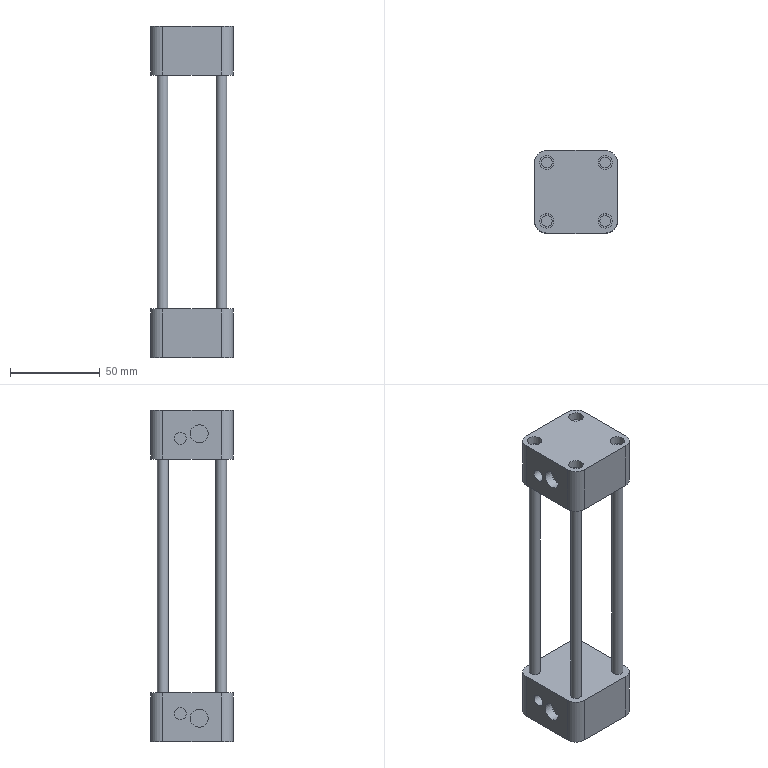Part | NX | features solid 2 | 1 solid | 48 faces | box 46 x 46 x 184 mm | volume 123684 mm3 | plane 24 | cylinder 24 | commonest cylinder face diameters 6 x8 13.5 x8 8 x4 6.667 x2 10 x2
STEP:
#1=CARTESIAN_POINT('',(-576.25,-3.,-304.));
#2=VERTEX_POINT('',#1);
#3=CARTESIAN_POINT('',(-543.75,-3.,-304.));
#4=VERTEX_POINT('',#3);
#5=CARTESIAN_POINT('',(-583.,-3.,-304.));
#6=DIRECTION('',(1.,0.,0.));
#7=VECTOR('',#6,1000.);
#8=LINE('',#5,#7);
#9=EDGE_CURVE('',#2,#4,#8,.T.);
#10=ORIENTED_EDGE('',*,*,#9,.F.);
#11=CARTESIAN_POINT('',(-576.25,-3.,-331.));
#12=VERTEX_POINT('',#11);
#13=CARTESIAN_POINT('',(-576.25,-3.,-331.));
#14=DIRECTION('',(0.,0.,-1.));
#15=VECTOR('',#14,1000.);
#16=LINE('',#13,#15);
#17=EDGE_CURVE('',#2,#12,#16,.T.);
#18=ORIENTED_EDGE('',*,*,#17,.T.);
#19=CARTESIAN_POINT('',(-543.75,-3.,-331.));
#20=VERTEX_POINT('',#19);
#21=CARTESIAN_POINT('',(-583.,-3.,-331.));
#22=DIRECTION('',(1.,0.,0.));
#23=VECTOR('',#22,1000.);
#24=LINE('',#21,#23);
#25=EDGE_CURVE('',#12,#20,#24,.T.);
#26=ORIENTED_EDGE('',*,*,#25,.T.);
#27=CARTESIAN_POINT('',(-543.75,-3.,-304.));
#28=DIRECTION('',(0.,0.,-1.));
#29=VECTOR('',#28,1000.);
#30=LINE('',#27,#29);
#31=EDGE_CURVE('',#20,#4,#30,.F.);
#32=ORIENTED_EDGE('',*,*,#31,.T.);
#33=EDGE_LOOP('',(#10,#18,#26,#32));
#34=FACE_BOUND('',#33,.T.);
#35=CARTESIAN_POINT('',(-583.,-3.,-304.));
#36=DIRECTION('',(0.,1.,0.));
#37=DIRECTION('',(-1.,0.,0.));
#38=AXIS2_PLACEMENT_3D('',#35,#36,#37);
#39=PLANE('',#38);
#40=ADVANCED_FACE('',(#34),#39,.F.);
#41=CARTESIAN_POINT('',(-537.,36.25,-304.));
#42=VERTEX_POINT('',#41);
#43=CARTESIAN_POINT('',(-537.,3.75,-304.));
#44=VERTEX_POINT('',#43);
#45=CARTESIAN_POINT('',(-537.,43.,-304.));
#46=DIRECTION('',(0.,-1.,0.));
#47=VECTOR('',#46,1000.);
#48=LINE('',#45,#47);
#49=EDGE_CURVE('',#42,#44,#48,.T.);
#50=ORIENTED_EDGE('',*,*,#49,.T.);
#51=CARTESIAN_POINT('',(-537.,3.75,-331.));
#52=VERTEX_POINT('',#51);
#53=CARTESIAN_POINT('',(-537.,3.75,-331.));
#54=DIRECTION('',(0.,0.,-1.));
#55=VECTOR('',#54,1000.);
#56=LINE('',#53,#55);
#57=EDGE_CURVE('',#44,#52,#56,.T.);
#58=ORIENTED_EDGE('',*,*,#57,.T.);
#59=CARTESIAN_POINT('',(-537.,36.25,-331.));
#60=VERTEX_POINT('',#59);
#61=CARTESIAN_POINT('',(-537.,43.,-331.));
#62=DIRECTION('',(0.,-1.,0.));
#63=VECTOR('',#62,1000.);
#64=LINE('',#61,#63);
#65=EDGE_CURVE('',#60,#52,#64,.T.);
#66=ORIENTED_EDGE('',*,*,#65,.F.);
#67=CARTESIAN_POINT('',(-537.,36.25,-304.));
#68=DIRECTION('',(0.,0.,-1.));
#69=VECTOR('',#68,1000.);
#70=LINE('',#67,#69);
#71=EDGE_CURVE('',#60,#42,#70,.F.);
#72=ORIENTED_EDGE('',*,*,#71,.T.);
#73=EDGE_LOOP('',(#50,#58,#66,#72));
#74=FACE_BOUND('',#73,.T.);
#75=CARTESIAN_POINT('',(-537.,43.,-304.));
#76=DIRECTION('',(1.,0.,0.));
#77=DIRECTION('',(0.,1.,0.));
#78=AXIS2_PLACEMENT_3D('',#75,#76,#77);
#79=PLANE('',#78);
#80=ADVANCED_FACE('',(#74),#79,.T.);
#81=CARTESIAN_POINT('',(-543.75,43.,-331.));
#82=VERTEX_POINT('',#81);
#83=CARTESIAN_POINT('',(-576.25,43.,-331.));
#84=VERTEX_POINT('',#83);
#85=CARTESIAN_POINT('',(-537.,43.,-331.));
#86=DIRECTION('',(-1.,0.,0.));
#87=VECTOR('',#86,1000.);
#88=LINE('',#85,#87);
#89=EDGE_CURVE('',#82,#84,#88,.T.);
#90=ORIENTED_EDGE('',*,*,#89,.T.);
#91=CARTESIAN_POINT('',(-576.25,43.,-304.));
#92=VERTEX_POINT('',#91);
#93=CARTESIAN_POINT('',(-576.25,43.,-304.));
#94=DIRECTION('',(0.,0.,-1.));
#95=VECTOR('',#94,1000.);
#96=LINE('',#93,#95);
#97=EDGE_CURVE('',#84,#92,#96,.F.);
#98=ORIENTED_EDGE('',*,*,#97,.T.);
#99=CARTESIAN_POINT('',(-543.75,43.,-304.));
#100=VERTEX_POINT('',#99);
#101=CARTESIAN_POINT('',(-537.,43.,-304.));
#102=DIRECTION('',(-1.,0.,0.));
#103=VECTOR('',#102,1000.);
#104=LINE('',#101,#103);
#105=EDGE_CURVE('',#100,#92,#104,.T.);
#106=ORIENTED_EDGE('',*,*,#105,.F.);
#107=CARTESIAN_POINT('',(-543.75,43.,-331.));
#108=DIRECTION('',(0.,0.,-1.));
#109=VECTOR('',#108,1000.);
#110=LINE('',#107,#109);
#111=EDGE_CURVE('',#100,#82,#110,.T.);
#112=ORIENTED_EDGE('',*,*,#111,.T.);
#113=EDGE_LOOP('',(#90,#98,#106,#112));
#114=FACE_BOUND('',#113,.T.);
#115=CARTESIAN_POINT('',(-537.,43.,-304.));
#116=DIRECTION('',(0.,-1.,0.));
#117=DIRECTION('',(1.,0.,0.));
#118=AXIS2_PLACEMENT_3D('',#115,#116,#117);
#119=PLANE('',#118);
#120=ADVANCED_FACE('',(#114),#119,.F.);
#121=CARTESIAN_POINT('',(-583.,26.5,-318.833));
#122=VERTEX_POINT('',#121);
#123=CARTESIAN_POINT('',(-583.,26.5,-315.5));
#124=DIRECTION('',(1.,0.,0.));
#125=DIRECTION('',(0.,0.,-1.));
#126=AXIS2_PLACEMENT_3D('',#123,#124,#125);
#127=CIRCLE('',#126,3.333);
#128=EDGE_CURVE('',#122,#122,#127,.T.);
#129=ORIENTED_EDGE('',*,*,#128,.T.);
#130=EDGE_LOOP('',(#129));
#131=FACE_BOUND('',#130,.T.);
#132=CARTESIAN_POINT('',(-583.,16.,-323.));
#133=VERTEX_POINT('',#132);
#134=CARTESIAN_POINT('',(-583.,16.,-318.));
#135=DIRECTION('',(1.,0.,0.));
#136=DIRECTION('',(0.,0.,-1.));
#137=AXIS2_PLACEMENT_3D('',#134,#135,#136);
#138=CIRCLE('',#137,5.);
#139=EDGE_CURVE('',#133,#133,#138,.T.);
#140=ORIENTED_EDGE('',*,*,#139,.T.);
#141=EDGE_LOOP('',(#140));
#142=FACE_BOUND('',#141,.T.);
#143=CARTESIAN_POINT('',(-583.,3.75,-331.));
#144=VERTEX_POINT('',#143);
#145=CARTESIAN_POINT('',(-583.,36.25,-331.));
#146=VERTEX_POINT('',#145);
#147=CARTESIAN_POINT('',(-583.,-3.,-331.));
#148=DIRECTION('',(0.,1.,0.));
#149=VECTOR('',#148,1000.);
#150=LINE('',#147,#149);
#151=EDGE_CURVE('',#144,#146,#150,.T.);
#152=ORIENTED_EDGE('',*,*,#151,.F.);
#153=CARTESIAN_POINT('',(-583.,3.75,-304.));
#154=VERTEX_POINT('',#153);
#155=CARTESIAN_POINT('',(-583.,3.75,-304.));
#156=DIRECTION('',(0.,0.,-1.));
#157=VECTOR('',#156,1000.);
#158=LINE('',#155,#157);
#159=EDGE_CURVE('',#144,#154,#158,.F.);
#160=ORIENTED_EDGE('',*,*,#159,.T.);
#161=CARTESIAN_POINT('',(-583.,36.25,-304.));
#162=VERTEX_POINT('',#161);
#163=CARTESIAN_POINT('',(-583.,-3.,-304.));
#164=DIRECTION('',(0.,1.,0.));
#165=VECTOR('',#164,1000.);
#166=LINE('',#163,#165);
#167=EDGE_CURVE('',#154,#162,#166,.T.);
#168=ORIENTED_EDGE('',*,*,#167,.T.);
#169=CARTESIAN_POINT('',(-583.,36.25,-331.));
#170=DIRECTION('',(0.,0.,-1.));
#171=VECTOR('',#170,1000.);
#172=LINE('',#169,#171);
#173=EDGE_CURVE('',#162,#146,#172,.T.);
#174=ORIENTED_EDGE('',*,*,#173,.T.);
#175=EDGE_LOOP('',(#152,#160,#168,#174));
#176=FACE_BOUND('',#175,.T.);
#177=CARTESIAN_POINT('',(-583.,-3.,-304.));
#178=DIRECTION('',(-1.,0.,0.));
#179=DIRECTION('',(0.,0.,1.));
#180=AXIS2_PLACEMENT_3D('',#177,#178,#179);
#181=PLANE('',#180);
#182=ADVANCED_FACE('',(#131,#142,#176),#181,.T.);
#183=CARTESIAN_POINT('',(-576.25,33.25,-304.));
#184=VERTEX_POINT('',#183);
#185=CARTESIAN_POINT('',(-576.25,36.25,-304.));
#186=DIRECTION('',(0.,0.,1.));
#187=DIRECTION('',(0.,-1.,0.));
#188=AXIS2_PLACEMENT_3D('',#185,#186,#187);
#189=CIRCLE('',#188,3.);
#190=EDGE_CURVE('',#184,#184,#189,.T.);
#191=ORIENTED_EDGE('',*,*,#190,.F.);
#192=EDGE_LOOP('',(#191));
#193=FACE_BOUND('',#192,.T.);
#194=CARTESIAN_POINT('',(-576.25,6.75,-304.));
#195=VERTEX_POINT('',#194);
#196=CARTESIAN_POINT('',(-576.25,3.75,-304.));
#197=DIRECTION('',(0.,0.,-1.));
#198=DIRECTION('',(0.,1.,0.));
#199=AXIS2_PLACEMENT_3D('',#196,#197,#198);
#200=CIRCLE('',#199,3.);
#201=EDGE_CURVE('',#195,#195,#200,.T.);
#202=ORIENTED_EDGE('',*,*,#201,.T.);
#203=EDGE_LOOP('',(#202));
#204=FACE_BOUND('',#203,.T.);
#205=CARTESIAN_POINT('',(-543.75,33.25,-304.));
#206=VERTEX_POINT('',#205);
#207=CARTESIAN_POINT('',(-543.75,36.25,-304.));
#208=DIRECTION('',(0.,0.,-1.));
#209=DIRECTION('',(0.,-1.,0.));
#210=AXIS2_PLACEMENT_3D('',#207,#208,#209);
#211=CIRCLE('',#210,3.);
#212=EDGE_CURVE('',#206,#206,#211,.T.);
#213=ORIENTED_EDGE('',*,*,#212,.T.);
#214=EDGE_LOOP('',(#213));
#215=FACE_BOUND('',#214,.T.);
#216=CARTESIAN_POINT('',(-543.75,6.75,-304.));
#217=VERTEX_POINT('',#216);
#218=CARTESIAN_POINT('',(-543.75,3.75,-304.));
#219=DIRECTION('',(0.,0.,1.));
#220=DIRECTION('',(0.,1.,0.));
#221=AXIS2_PLACEMENT_3D('',#218,#219,#220);
#222=CIRCLE('',#221,3.);
#223=EDGE_CURVE('',#217,#217,#222,.T.);
#224=ORIENTED_EDGE('',*,*,#223,.F.);
#225=EDGE_LOOP('',(#224));
#226=FACE_BOUND('',#225,.T.);
#227=ORIENTED_EDGE('',*,*,#167,.F.);
#228=CARTESIAN_POINT('',(-576.25,3.75,-304.));
#229=DIRECTION('',(0.,0.,-1.));
#230=DIRECTION('',(0.,-1.,0.));
#231=AXIS2_PLACEMENT_3D('',#228,#229,#230);
#232=CIRCLE('',#231,6.75);
#233=EDGE_CURVE('',#154,#2,#232,.F.);
#234=ORIENTED_EDGE('',*,*,#233,.T.);
#235=ORIENTED_EDGE('',*,*,#9,.T.);
#236=CARTESIAN_POINT('',(-543.75,3.75,-304.));
#237=DIRECTION('',(0.,0.,-1.));
#238=DIRECTION('',(0.,-1.,0.));
#239=AXIS2_PLACEMENT_3D('',#236,#237,#238);
#240=CIRCLE('',#239,6.75);
#241=EDGE_CURVE('',#4,#44,#240,.F.);
#242=ORIENTED_EDGE('',*,*,#241,.T.);
#243=ORIENTED_EDGE('',*,*,#49,.F.);
#244=CARTESIAN_POINT('',(-543.75,36.25,-304.));
#245=DIRECTION('',(0.,0.,-1.));
#246=DIRECTION('',(0.,-1.,0.));
#247=AXIS2_PLACEMENT_3D('',#244,#245,#246);
#248=CIRCLE('',#247,6.75);
#249=EDGE_CURVE('',#42,#100,#248,.F.);
#250=ORIENTED_EDGE('',*,*,#249,.T.);
#251=ORIENTED_EDGE('',*,*,#105,.T.);
#252=CARTESIAN_POINT('',(-576.25,36.25,-304.));
#253=DIRECTION('',(0.,0.,-1.));
#254=DIRECTION('',(0.,-1.,0.));
#255=AXIS2_PLACEMENT_3D('',#252,#253,#254);
#256=CIRCLE('',#255,6.75);
#257=EDGE_CURVE('',#92,#162,#256,.F.);
#258=ORIENTED_EDGE('',*,*,#257,.T.);
#259=EDGE_LOOP('',(#227,#234,#235,#242,#243,#250,#251,#258));
#260=FACE_BOUND('',#259,.T.);
#261=CARTESIAN_POINT('',(-537.,-3.,-304.));
#262=DIRECTION('',(0.,0.,-1.));
#263=DIRECTION('',(0.,-1.,0.));
#264=AXIS2_PLACEMENT_3D('',#261,#262,#263);
#265=PLANE('',#264);
#266=ADVANCED_FACE('',(#193,#204,#215,#226,#260),#265,.F.);
#267=ORIENTED_EDGE('',*,*,#25,.F.);
#268=CARTESIAN_POINT('',(-576.25,3.75,-331.));
#269=DIRECTION('',(0.,0.,-1.));
#270=DIRECTION('',(0.,-1.,0.));
#271=AXIS2_PLACEMENT_3D('',#268,#269,#270);
#272=CIRCLE('',#271,6.75);
#273=EDGE_CURVE('',#12,#144,#272,.T.);
#274=ORIENTED_EDGE('',*,*,#273,.T.);
#275=ORIENTED_EDGE('',*,*,#151,.T.);
#276=CARTESIAN_POINT('',(-576.25,36.25,-331.));
#277=DIRECTION('',(0.,0.,-1.));
#278=DIRECTION('',(0.,-1.,0.));
#279=AXIS2_PLACEMENT_3D('',#276,#277,#278);
#280=CIRCLE('',#279,6.75);
#281=EDGE_CURVE('',#146,#84,#280,.T.);
#282=ORIENTED_EDGE('',*,*,#281,.T.);
#283=ORIENTED_EDGE('',*,*,#89,.F.);
#284=CARTESIAN_POINT('',(-543.75,36.25,-331.));
#285=DIRECTION('',(0.,0.,-1.));
#286=DIRECTION('',(0.,-1.,0.));
#287=AXIS2_PLACEMENT_3D('',#284,#285,#286);
#288=CIRCLE('',#287,6.75);
#289=EDGE_CURVE('',#82,#60,#288,.T.);
#290=ORIENTED_EDGE('',*,*,#289,.T.);
#291=ORIENTED_EDGE('',*,*,#65,.T.);
#292=CARTESIAN_POINT('',(-543.75,3.75,-331.));
#293=DIRECTION('',(0.,0.,-1.));
#294=DIRECTION('',(0.,-1.,0.));
#295=AXIS2_PLACEMENT_3D('',#292,#293,#294);
#296=CIRCLE('',#295,6.75);
#297=EDGE_CURVE('',#52,#20,#296,.T.);
#298=ORIENTED_EDGE('',*,*,#297,.T.);
#299=EDGE_LOOP('',(#267,#274,#275,#282,#283,#290,#291,#298));
#300=FACE_BOUND('',#299,.T.);
#301=CARTESIAN_POINT('',(-537.,-3.,-331.));
#302=DIRECTION('',(0.,0.,-1.));
#303=DIRECTION('',(0.,-1.,0.));
#304=AXIS2_PLACEMENT_3D('',#301,#302,#303);
#305=PLANE('',#304);
#306=ADVANCED_FACE('',(#300),#305,.T.);
#307=ORIENTED_EDGE('',*,*,#233,.F.);
#308=ORIENTED_EDGE('',*,*,#159,.F.);
#309=ORIENTED_EDGE('',*,*,#273,.F.);
#310=ORIENTED_EDGE('',*,*,#17,.F.);
#311=EDGE_LOOP('',(#307,#308,#309,#310));
#312=FACE_BOUND('',#311,.T.);
#313=CARTESIAN_POINT('',(-576.25,3.75,-304.));
#314=DIRECTION('',(0.,0.,1.));
#315=DIRECTION('',(0.,1.,0.));
#316=AXIS2_PLACEMENT_3D('',#313,#314,#315);
#317=CYLINDRICAL_SURFACE('',#316,6.75);
#318=ADVANCED_FACE('',(#312),#317,.T.);
#319=ORIENTED_EDGE('',*,*,#241,.F.);
#320=ORIENTED_EDGE('',*,*,#31,.F.);
#321=ORIENTED_EDGE('',*,*,#297,.F.);
#322=ORIENTED_EDGE('',*,*,#57,.F.);
#323=EDGE_LOOP('',(#319,#320,#321,#322));
#324=FACE_BOUND('',#323,.T.);
#325=CARTESIAN_POINT('',(-543.75,3.75,-304.));
#326=DIRECTION('',(0.,0.,1.));
#327=DIRECTION('',(0.,1.,0.));
#328=AXIS2_PLACEMENT_3D('',#325,#326,#327);
#329=CYLINDRICAL_SURFACE('',#328,6.75);
#330=ADVANCED_FACE('',(#324),#329,.T.);
#331=ORIENTED_EDGE('',*,*,#257,.F.);
#332=ORIENTED_EDGE('',*,*,#97,.F.);
#333=ORIENTED_EDGE('',*,*,#281,.F.);
#334=ORIENTED_EDGE('',*,*,#173,.F.);
#335=EDGE_LOOP('',(#331,#332,#333,#334));
#336=FACE_BOUND('',#335,.T.);
#337=CARTESIAN_POINT('',(-576.25,36.25,-304.));
#338=DIRECTION('',(0.,0.,1.));
#339=DIRECTION('',(0.,1.,0.));
#340=AXIS2_PLACEMENT_3D('',#337,#338,#339);
#341=CYLINDRICAL_SURFACE('',#340,6.75);
#342=ADVANCED_FACE('',(#336),#341,.T.);
#343=ORIENTED_EDGE('',*,*,#249,.F.);
#344=ORIENTED_EDGE('',*,*,#71,.F.);
#345=ORIENTED_EDGE('',*,*,#289,.F.);
#346=ORIENTED_EDGE('',*,*,#111,.F.);
#347=EDGE_LOOP('',(#343,#344,#345,#346));
#348=FACE_BOUND('',#347,.T.);
#349=CARTESIAN_POINT('',(-543.75,36.25,-304.));
#350=DIRECTION('',(0.,0.,1.));
#351=DIRECTION('',(0.,1.,0.));
#352=AXIS2_PLACEMENT_3D('',#349,#350,#351);
#353=CYLINDRICAL_SURFACE('',#352,6.75);
#354=ADVANCED_FACE('',(#348),#353,.T.);
#355=CARTESIAN_POINT('',(-543.75,0.75,-174.));
#356=VERTEX_POINT('',#355);
#357=CARTESIAN_POINT('',(-543.75,3.75,-174.));
#358=DIRECTION('',(0.,0.,-1.));
#359=DIRECTION('',(0.,-1.,0.));
#360=AXIS2_PLACEMENT_3D('',#357,#358,#359);
#361=CIRCLE('',#360,3.);
#362=EDGE_CURVE('',#356,#356,#361,.F.);
#363=ORIENTED_EDGE('',*,*,#362,.F.);
#364=EDGE_LOOP('',(#363));
#365=FACE_BOUND('',#364,.T.);
#366=ORIENTED_EDGE('',*,*,#223,.T.);
#367=EDGE_LOOP('',(#366));
#368=FACE_BOUND('',#367,.T.);
#369=CARTESIAN_POINT('',(-543.75,3.75,-304.));
#370=DIRECTION('',(0.,0.,1.));
#371=DIRECTION('',(0.,1.,0.));
#372=AXIS2_PLACEMENT_3D('',#369,#370,#371);
#373=CYLINDRICAL_SURFACE('',#372,3.);
#374=ADVANCED_FACE('',(#365,#368),#373,.T.);
#375=CARTESIAN_POINT('',(-543.75,33.25,-174.));
#376=VERTEX_POINT('',#375);
#377=CARTESIAN_POINT('',(-543.75,36.25,-174.));
#378=DIRECTION('',(0.,0.,-1.));
#379=DIRECTION('',(0.,-1.,0.));
#380=AXIS2_PLACEMENT_3D('',#377,#378,#379);
#381=CIRCLE('',#380,3.);
#382=EDGE_CURVE('',#376,#376,#381,.F.);
#383=ORIENTED_EDGE('',*,*,#382,.F.);
#384=EDGE_LOOP('',(#383));
#385=FACE_BOUND('',#384,.T.);
#386=ORIENTED_EDGE('',*,*,#212,.F.);
#387=EDGE_LOOP('',(#386));
#388=FACE_BOUND('',#387,.T.);
#389=CARTESIAN_POINT('',(-543.75,36.25,-304.));
#390=DIRECTION('',(0.,0.,1.));
#391=DIRECTION('',(0.,-1.,0.));
#392=AXIS2_PLACEMENT_3D('',#389,#390,#391);
#393=CYLINDRICAL_SURFACE('',#392,3.);
#394=ADVANCED_FACE('',(#385,#388),#393,.T.);
#395=CARTESIAN_POINT('',(-576.25,0.75,-174.));
#396=VERTEX_POINT('',#395);
#397=CARTESIAN_POINT('',(-576.25,3.75,-174.));
#398=DIRECTION('',(0.,0.,-1.));
#399=DIRECTION('',(0.,-1.,0.));
#400=AXIS2_PLACEMENT_3D('',#397,#398,#399);
#401=CIRCLE('',#400,3.);
#402=EDGE_CURVE('',#396,#396,#401,.F.);
#403=ORIENTED_EDGE('',*,*,#402,.F.);
#404=EDGE_LOOP('',(#403));
#405=FACE_BOUND('',#404,.T.);
#406=ORIENTED_EDGE('',*,*,#201,.F.);
#407=EDGE_LOOP('',(#406));
#408=FACE_BOUND('',#407,.T.);
#409=CARTESIAN_POINT('',(-576.25,3.75,-304.));
#410=DIRECTION('',(0.,0.,1.));
#411=DIRECTION('',(0.,1.,0.));
#412=AXIS2_PLACEMENT_3D('',#409,#410,#411);
#413=CYLINDRICAL_SURFACE('',#412,3.);
#414=ADVANCED_FACE('',(#405,#408),#413,.T.);
#415=CARTESIAN_POINT('',(-576.25,33.25,-174.));
#416=VERTEX_POINT('',#415);
#417=CARTESIAN_POINT('',(-576.25,36.25,-174.));
#418=DIRECTION('',(0.,0.,-1.));
#419=DIRECTION('',(0.,-1.,0.));
#420=AXIS2_PLACEMENT_3D('',#417,#418,#419);
#421=CIRCLE('',#420,3.);
#422=EDGE_CURVE('',#416,#416,#421,.F.);
#423=ORIENTED_EDGE('',*,*,#422,.F.);
#424=EDGE_LOOP('',(#423));
#425=FACE_BOUND('',#424,.T.);
#426=ORIENTED_EDGE('',*,*,#190,.T.);
#427=EDGE_LOOP('',(#426));
#428=FACE_BOUND('',#427,.T.);
#429=CARTESIAN_POINT('',(-576.25,36.25,-304.));
#430=DIRECTION('',(0.,0.,1.));
#431=DIRECTION('',(0.,-1.,0.));
#432=AXIS2_PLACEMENT_3D('',#429,#430,#431);
#433=CYLINDRICAL_SURFACE('',#432,3.);
#434=ADVANCED_FACE('',(#425,#428),#433,.T.);
#435=CARTESIAN_POINT('',(-578.,16.,-323.));
#436=VERTEX_POINT('',#435);
#437=CARTESIAN_POINT('',(-578.,16.,-318.));
#438=DIRECTION('',(1.,0.,0.));
#439=DIRECTION('',(0.,0.,-1.));
#440=AXIS2_PLACEMENT_3D('',#437,#438,#439);
#441=CIRCLE('',#440,5.);
#442=EDGE_CURVE('',#436,#436,#441,.T.);
#443=ORIENTED_EDGE('',*,*,#442,.F.);
#444=EDGE_LOOP('',(#443));
#445=FACE_BOUND('',#444,.T.);
#446=CARTESIAN_POINT('',(-578.,16.,-318.));
#447=DIRECTION('',(1.,0.,0.));
#448=DIRECTION('',(0.,0.,-1.));
#449=AXIS2_PLACEMENT_3D('',#446,#447,#448);
#450=PLANE('',#449);
#451=ADVANCED_FACE('',(#445),#450,.F.);
#452=ORIENTED_EDGE('',*,*,#442,.T.);
#453=EDGE_LOOP('',(#452));
#454=FACE_BOUND('',#453,.T.);
#455=ORIENTED_EDGE('',*,*,#139,.F.);
#456=EDGE_LOOP('',(#455));
#457=FACE_BOUND('',#456,.T.);
#458=CARTESIAN_POINT('',(-583.,16.,-318.));
#459=DIRECTION('',(1.,0.,0.));
#460=DIRECTION('',(0.,0.,-1.));
#461=AXIS2_PLACEMENT_3D('',#458,#459,#460);
#462=CYLINDRICAL_SURFACE('',#461,5.);
#463=ADVANCED_FACE('',(#454,#457),#462,.F.);
#464=CARTESIAN_POINT('',(-578.,26.5,-318.833));
#465=VERTEX_POINT('',#464);
#466=CARTESIAN_POINT('',(-578.,26.5,-315.5));
#467=DIRECTION('',(1.,0.,0.));
#468=DIRECTION('',(0.,0.,-1.));
#469=AXIS2_PLACEMENT_3D('',#466,#467,#468);
#470=CIRCLE('',#469,3.333);
#471=EDGE_CURVE('',#465,#465,#470,.T.);
#472=ORIENTED_EDGE('',*,*,#471,.F.);
#473=EDGE_LOOP('',(#472));
#474=FACE_BOUND('',#473,.T.);
#475=CARTESIAN_POINT('',(-578.,26.5,-315.5));
#476=DIRECTION('',(1.,0.,0.));
#477=DIRECTION('',(0.,0.,-1.));
#478=AXIS2_PLACEMENT_3D('',#475,#476,#477);
#479=PLANE('',#478);
#480=ADVANCED_FACE('',(#474),#479,.F.);
#481=ORIENTED_EDGE('',*,*,#471,.T.);
#482=EDGE_LOOP('',(#481));
#483=FACE_BOUND('',#482,.T.);
#484=ORIENTED_EDGE('',*,*,#128,.F.);
#485=EDGE_LOOP('',(#484));
#486=FACE_BOUND('',#485,.T.);
#487=CARTESIAN_POINT('',(-583.,26.5,-315.5));
#488=DIRECTION('',(1.,0.,0.));
#489=DIRECTION('',(0.,0.,-1.));
#490=AXIS2_PLACEMENT_3D('',#487,#488,#489);
#491=CYLINDRICAL_SURFACE('',#490,3.333);
#492=ADVANCED_FACE('',(#483,#486),#491,.F.);
#493=CARTESIAN_POINT('',(-543.75,43.,-174.));
#494=VERTEX_POINT('',#493);
#495=CARTESIAN_POINT('',(-576.25,43.,-174.));
#496=VERTEX_POINT('',#495);
#497=CARTESIAN_POINT('',(-537.,43.,-174.));
#498=DIRECTION('',(-1.,0.,0.));
#499=VECTOR('',#498,1000.);
#500=LINE('',#497,#499);
#501=EDGE_CURVE('',#494,#496,#500,.T.);
#502=ORIENTED_EDGE('',*,*,#501,.T.);
#503=CARTESIAN_POINT('',(-576.25,43.,-147.));
#504=VERTEX_POINT('',#503);
#505=CARTESIAN_POINT('',(-576.25,43.,-147.));
#506=DIRECTION('',(0.,0.,1.));
#507=VECTOR('',#506,1000.);
#508=LINE('',#505,#507);
#509=EDGE_CURVE('',#496,#504,#508,.T.);
#510=ORIENTED_EDGE('',*,*,#509,.T.);
#511=CARTESIAN_POINT('',(-543.75,43.,-147.));
#512=VERTEX_POINT('',#511);
#513=CARTESIAN_POINT('',(-537.,43.,-147.));
#514=DIRECTION('',(-1.,0.,0.));
#515=VECTOR('',#514,1000.);
#516=LINE('',#513,#515);
#517=EDGE_CURVE('',#512,#504,#516,.T.);
#518=ORIENTED_EDGE('',*,*,#517,.F.);
#519=CARTESIAN_POINT('',(-543.75,43.,-174.));
#520=DIRECTION('',(0.,0.,1.));
#521=VECTOR('',#520,1000.);
#522=LINE('',#519,#521);
#523=EDGE_CURVE('',#512,#494,#522,.F.);
#524=ORIENTED_EDGE('',*,*,#523,.T.);
#525=EDGE_LOOP('',(#502,#510,#518,#524));
#526=FACE_BOUND('',#525,.T.);
#527=CARTESIAN_POINT('',(-537.,43.,-174.));
#528=DIRECTION('',(0.,1.,0.));
#529=DIRECTION('',(-1.,0.,0.));
#530=AXIS2_PLACEMENT_3D('',#527,#528,#529);
#531=PLANE('',#530);
#532=ADVANCED_FACE('',(#526),#531,.T.);
#533=CARTESIAN_POINT('',(-583.,26.5,-165.833));
#534=VERTEX_POINT('',#533);
#535=CARTESIAN_POINT('',(-583.,26.5,-162.5));
#536=DIRECTION('',(1.,0.,0.));
#537=DIRECTION('',(0.,0.,-1.));
#538=AXIS2_PLACEMENT_3D('',#535,#536,#537);
#539=CIRCLE('',#538,3.333);
#540=EDGE_CURVE('',#534,#534,#539,.T.);
#541=ORIENTED_EDGE('',*,*,#540,.T.);
#542=EDGE_LOOP('',(#541));
#543=FACE_BOUND('',#542,.T.);
#544=CARTESIAN_POINT('',(-583.,16.,-165.));
#545=VERTEX_POINT('',#544);
#546=CARTESIAN_POINT('',(-583.,16.,-160.));
#547=DIRECTION('',(1.,0.,0.));
#548=DIRECTION('',(0.,0.,-1.));
#549=AXIS2_PLACEMENT_3D('',#546,#547,#548);
#550=CIRCLE('',#549,5.);
#551=EDGE_CURVE('',#545,#545,#550,.T.);
#552=ORIENTED_EDGE('',*,*,#551,.T.);
#553=EDGE_LOOP('',(#552));
#554=FACE_BOUND('',#553,.T.);
#555=CARTESIAN_POINT('',(-583.,3.75,-147.));
#556=VERTEX_POINT('',#555);
#557=CARTESIAN_POINT('',(-583.,36.25,-147.));
#558=VERTEX_POINT('',#557);
#559=CARTESIAN_POINT('',(-583.,-3.,-147.));
#560=DIRECTION('',(0.,1.,0.));
#561=VECTOR('',#560,1000.);
#562=LINE('',#559,#561);
#563=EDGE_CURVE('',#556,#558,#562,.T.);
#564=ORIENTED_EDGE('',*,*,#563,.T.);
#565=CARTESIAN_POINT('',(-583.,36.25,-174.));
#566=VERTEX_POINT('',#565);
#567=CARTESIAN_POINT('',(-583.,36.25,-174.));
#568=DIRECTION('',(0.,0.,1.));
#569=VECTOR('',#568,1000.);
#570=LINE('',#567,#569);
#571=EDGE_CURVE('',#558,#566,#570,.F.);
#572=ORIENTED_EDGE('',*,*,#571,.T.);
#573=CARTESIAN_POINT('',(-583.,3.75,-174.));
#574=VERTEX_POINT('',#573);
#575=CARTESIAN_POINT('',(-583.,-3.,-174.));
#576=DIRECTION('',(0.,1.,0.));
#577=VECTOR('',#576,1000.);
#578=LINE('',#575,#577);
#579=EDGE_CURVE('',#574,#566,#578,.T.);
#580=ORIENTED_EDGE('',*,*,#579,.F.);
#581=CARTESIAN_POINT('',(-583.,3.75,-147.));
#582=DIRECTION('',(0.,0.,1.));
#583=VECTOR('',#582,1000.);
#584=LINE('',#581,#583);
#585=EDGE_CURVE('',#574,#556,#584,.T.);
#586=ORIENTED_EDGE('',*,*,#585,.T.);
#587=EDGE_LOOP('',(#564,#572,#580,#586));
#588=FACE_BOUND('',#587,.T.);
#589=CARTESIAN_POINT('',(-583.,-3.,-174.));
#590=DIRECTION('',(1.,0.,0.));
#591=DIRECTION('',(0.,0.,-1.));
#592=AXIS2_PLACEMENT_3D('',#589,#590,#591);
#593=PLANE('',#592);
#594=ADVANCED_FACE('',(#543,#554,#588),#593,.F.);
#595=CARTESIAN_POINT('',(-576.25,-3.,-174.));
#596=VERTEX_POINT('',#595);
#597=CARTESIAN_POINT('',(-543.75,-3.,-174.));
#598=VERTEX_POINT('',#597);
#599=CARTESIAN_POINT('',(-583.,-3.,-174.));
#600=DIRECTION('',(1.,0.,0.));
#601=VECTOR('',#600,1000.);
#602=LINE('',#599,#601);
#603=EDGE_CURVE('',#596,#598,#602,.T.);
#604=ORIENTED_EDGE('',*,*,#603,.T.);
#605=CARTESIAN_POINT('',(-543.75,-3.,-147.));
#606=VERTEX_POINT('',#605);
#607=CARTESIAN_POINT('',(-543.75,-3.,-147.));
#608=DIRECTION('',(0.,0.,1.));
#609=VECTOR('',#608,1000.);
#610=LINE('',#607,#609);
#611=EDGE_CURVE('',#598,#606,#610,.T.);
#612=ORIENTED_EDGE('',*,*,#611,.T.);
#613=CARTESIAN_POINT('',(-576.25,-3.,-147.));
#614=VERTEX_POINT('',#613);
#615=CARTESIAN_POINT('',(-583.,-3.,-147.));
#616=DIRECTION('',(1.,0.,0.));
#617=VECTOR('',#616,1000.);
#618=LINE('',#615,#617);
#619=EDGE_CURVE('',#614,#606,#618,.T.);
#620=ORIENTED_EDGE('',*,*,#619,.F.);
#621=CARTESIAN_POINT('',(-576.25,-3.,-174.));
#622=DIRECTION('',(0.,0.,1.));
#623=VECTOR('',#622,1000.);
#624=LINE('',#621,#623);
#625=EDGE_CURVE('',#614,#596,#624,.F.);
#626=ORIENTED_EDGE('',*,*,#625,.T.);
#627=EDGE_LOOP('',(#604,#612,#620,#626));
#628=FACE_BOUND('',#627,.T.);
#629=CARTESIAN_POINT('',(-583.,-3.,-174.));
#630=DIRECTION('',(0.,-1.,0.));
#631=DIRECTION('',(1.,0.,0.));
#632=AXIS2_PLACEMENT_3D('',#629,#630,#631);
#633=PLANE('',#632);
#634=ADVANCED_FACE('',(#628),#633,.T.);
#635=CARTESIAN_POINT('',(-537.,36.25,-174.));
#636=VERTEX_POINT('',#635);
#637=CARTESIAN_POINT('',(-537.,3.75,-174.));
#638=VERTEX_POINT('',#637);
#639=CARTESIAN_POINT('',(-537.,43.,-174.));
#640=DIRECTION('',(0.,-1.,0.));
#641=VECTOR('',#640,1000.);
#642=LINE('',#639,#641);
#643=EDGE_CURVE('',#636,#638,#642,.T.);
#644=ORIENTED_EDGE('',*,*,#643,.F.);
#645=CARTESIAN_POINT('',(-537.,36.25,-147.));
#646=VERTEX_POINT('',#645);
#647=CARTESIAN_POINT('',(-537.,36.25,-147.));
#648=DIRECTION('',(0.,0.,1.));
#649=VECTOR('',#648,1000.);
#650=LINE('',#647,#649);
#651=EDGE_CURVE('',#636,#646,#650,.T.);
#652=ORIENTED_EDGE('',*,*,#651,.T.);
#653=CARTESIAN_POINT('',(-537.,3.75,-147.));
#654=VERTEX_POINT('',#653);
#655=CARTESIAN_POINT('',(-537.,43.,-147.));
#656=DIRECTION('',(0.,-1.,0.));
#657=VECTOR('',#656,1000.);
#658=LINE('',#655,#657);
#659=EDGE_CURVE('',#646,#654,#658,.T.);
#660=ORIENTED_EDGE('',*,*,#659,.T.);
#661=CARTESIAN_POINT('',(-537.,3.75,-174.));
#662=DIRECTION('',(0.,0.,1.));
#663=VECTOR('',#662,1000.);
#664=LINE('',#661,#663);
#665=EDGE_CURVE('',#654,#638,#664,.F.);
#666=ORIENTED_EDGE('',*,*,#665,.T.);
#667=EDGE_LOOP('',(#644,#652,#660,#666));
#668=FACE_BOUND('',#667,.T.);
#669=CARTESIAN_POINT('',(-537.,43.,-174.));
#670=DIRECTION('',(-1.,0.,0.));
#671=DIRECTION('',(0.,-1.,0.));
#672=AXIS2_PLACEMENT_3D('',#669,#670,#671);
#673=PLANE('',#672);
#674=ADVANCED_FACE('',(#668),#673,.F.);
#675=ORIENTED_EDGE('',*,*,#362,.T.);
#676=EDGE_LOOP('',(#675));
#677=FACE_BOUND('',#676,.T.);
#678=ORIENTED_EDGE('',*,*,#382,.T.);
#679=EDGE_LOOP('',(#678));
#680=FACE_BOUND('',#679,.T.);
#681=ORIENTED_EDGE('',*,*,#402,.T.);
#682=EDGE_LOOP('',(#681));
#683=FACE_BOUND('',#682,.T.);
#684=ORIENTED_EDGE('',*,*,#422,.T.);
#685=EDGE_LOOP('',(#684));
#686=FACE_BOUND('',#685,.T.);
#687=ORIENTED_EDGE('',*,*,#579,.T.);
#688=CARTESIAN_POINT('',(-576.25,36.25,-174.));
#689=DIRECTION('',(0.,0.,-1.));
#690=DIRECTION('',(0.,-1.,0.));
#691=AXIS2_PLACEMENT_3D('',#688,#689,#690);
#692=CIRCLE('',#691,6.75);
#693=EDGE_CURVE('',#566,#496,#692,.T.);
#694=ORIENTED_EDGE('',*,*,#693,.T.);
#695=ORIENTED_EDGE('',*,*,#501,.F.);
#696=CARTESIAN_POINT('',(-543.75,36.25,-174.));
#697=DIRECTION('',(0.,0.,-1.));
#698=DIRECTION('',(0.,-1.,0.));
#699=AXIS2_PLACEMENT_3D('',#696,#697,#698);
#700=CIRCLE('',#699,6.75);
#701=EDGE_CURVE('',#494,#636,#700,.T.);
#702=ORIENTED_EDGE('',*,*,#701,.T.);
#703=ORIENTED_EDGE('',*,*,#643,.T.);
#704=CARTESIAN_POINT('',(-543.75,3.75,-174.));
#705=DIRECTION('',(0.,0.,-1.));
#706=DIRECTION('',(0.,-1.,0.));
#707=AXIS2_PLACEMENT_3D('',#704,#705,#706);
#708=CIRCLE('',#707,6.75);
#709=EDGE_CURVE('',#638,#598,#708,.T.);
#710=ORIENTED_EDGE('',*,*,#709,.T.);
#711=ORIENTED_EDGE('',*,*,#603,.F.);
#712=CARTESIAN_POINT('',(-576.25,3.75,-174.));
#713=DIRECTION('',(0.,0.,-1.));
#714=DIRECTION('',(0.,-1.,0.));
#715=AXIS2_PLACEMENT_3D('',#712,#713,#714);
#716=CIRCLE('',#715,6.75);
#717=EDGE_CURVE('',#596,#574,#716,.T.);
#718=ORIENTED_EDGE('',*,*,#717,.T.);
#719=EDGE_LOOP('',(#687,#694,#695,#702,#703,#710,#711,#718));
#720=FACE_BOUND('',#719,.T.);
#721=CARTESIAN_POINT('',(-583.,43.,-174.));
#722=DIRECTION('',(0.,0.,-1.));
#723=DIRECTION('',(0.,-1.,0.));
#724=AXIS2_PLACEMENT_3D('',#721,#722,#723);
#725=PLANE('',#724);
#726=ADVANCED_FACE('',(#677,#680,#683,#686,#720),#725,.T.);
#727=CARTESIAN_POINT('',(-543.75,7.75,-147.));
#728=VERTEX_POINT('',#727);
#729=CARTESIAN_POINT('',(-543.75,3.75,-147.));
#730=DIRECTION('',(0.,0.,-1.));
#731=DIRECTION('',(0.,1.,0.));
#732=AXIS2_PLACEMENT_3D('',#729,#730,#731);
#733=CIRCLE('',#732,4.);
#734=EDGE_CURVE('',#728,#728,#733,.T.);
#735=ORIENTED_EDGE('',*,*,#734,.T.);
#736=EDGE_LOOP('',(#735));
#737=FACE_BOUND('',#736,.T.);
#738=CARTESIAN_POINT('',(-576.25,7.75,-147.));
#739=VERTEX_POINT('',#738);
#740=CARTESIAN_POINT('',(-576.25,3.75,-147.));
#741=DIRECTION('',(0.,0.,1.));
#742=DIRECTION('',(0.,1.,0.));
#743=AXIS2_PLACEMENT_3D('',#740,#741,#742);
#744=CIRCLE('',#743,4.);
#745=EDGE_CURVE('',#739,#739,#744,.T.);
#746=ORIENTED_EDGE('',*,*,#745,.F.);
#747=EDGE_LOOP('',(#746));
#748=FACE_BOUND('',#747,.T.);
#749=CARTESIAN_POINT('',(-543.75,32.25,-147.));
#750=VERTEX_POINT('',#749);
#751=CARTESIAN_POINT('',(-543.75,36.25,-147.));
#752=DIRECTION('',(0.,0.,1.));
#753=DIRECTION('',(0.,-1.,0.));
#754=AXIS2_PLACEMENT_3D('',#751,#752,#753);
#755=CIRCLE('',#754,4.);
#756=EDGE_CURVE('',#750,#750,#755,.T.);
#757=ORIENTED_EDGE('',*,*,#756,.F.);
#758=EDGE_LOOP('',(#757));
#759=FACE_BOUND('',#758,.T.);
#760=CARTESIAN_POINT('',(-576.25,32.25,-147.));
#761=VERTEX_POINT('',#760);
#762=CARTESIAN_POINT('',(-576.25,36.25,-147.));
#763=DIRECTION('',(0.,0.,-1.));
#764=DIRECTION('',(0.,-1.,0.));
#765=AXIS2_PLACEMENT_3D('',#762,#763,#764);
#766=CIRCLE('',#765,4.);
#767=EDGE_CURVE('',#761,#761,#766,.T.);
#768=ORIENTED_EDGE('',*,*,#767,.T.);
#769=EDGE_LOOP('',(#768));
#770=FACE_BOUND('',#769,.T.);
#771=ORIENTED_EDGE('',*,*,#517,.T.);
#772=CARTESIAN_POINT('',(-576.25,36.25,-147.));
#773=DIRECTION('',(0.,0.,-1.));
#774=DIRECTION('',(0.,-1.,0.));
#775=AXIS2_PLACEMENT_3D('',#772,#773,#774);
#776=CIRCLE('',#775,6.75);
#777=EDGE_CURVE('',#504,#558,#776,.F.);
#778=ORIENTED_EDGE('',*,*,#777,.T.);
#779=ORIENTED_EDGE('',*,*,#563,.F.);
#780=CARTESIAN_POINT('',(-576.25,3.75,-147.));
#781=DIRECTION('',(0.,0.,-1.));
#782=DIRECTION('',(0.,-1.,0.));
#783=AXIS2_PLACEMENT_3D('',#780,#781,#782);
#784=CIRCLE('',#783,6.75);
#785=EDGE_CURVE('',#556,#614,#784,.F.);
#786=ORIENTED_EDGE('',*,*,#785,.T.);
#787=ORIENTED_EDGE('',*,*,#619,.T.);
#788=CARTESIAN_POINT('',(-543.75,3.75,-147.));
#789=DIRECTION('',(0.,0.,-1.));
#790=DIRECTION('',(0.,-1.,0.));
#791=AXIS2_PLACEMENT_3D('',#788,#789,#790);
#792=CIRCLE('',#791,6.75);
#793=EDGE_CURVE('',#606,#654,#792,.F.);
#794=ORIENTED_EDGE('',*,*,#793,.T.);
#795=ORIENTED_EDGE('',*,*,#659,.F.);
#796=CARTESIAN_POINT('',(-543.75,36.25,-147.));
#797=DIRECTION('',(0.,0.,-1.));
#798=DIRECTION('',(0.,-1.,0.));
#799=AXIS2_PLACEMENT_3D('',#796,#797,#798);
#800=CIRCLE('',#799,6.75);
#801=EDGE_CURVE('',#646,#512,#800,.F.);
#802=ORIENTED_EDGE('',*,*,#801,.T.);
#803=EDGE_LOOP('',(#771,#778,#779,#786,#787,#794,#795,#802));
#804=FACE_BOUND('',#803,.T.);
#805=CARTESIAN_POINT('',(-583.,43.,-147.));
#806=DIRECTION('',(0.,0.,-1.));
#807=DIRECTION('',(0.,-1.,0.));
#808=AXIS2_PLACEMENT_3D('',#805,#806,#807);
#809=PLANE('',#808);
#810=ADVANCED_FACE('',(#737,#748,#759,#770,#804),#809,.F.);
#811=ORIENTED_EDGE('',*,*,#693,.F.);
#812=ORIENTED_EDGE('',*,*,#571,.F.);
#813=ORIENTED_EDGE('',*,*,#777,.F.);
#814=ORIENTED_EDGE('',*,*,#509,.F.);
#815=EDGE_LOOP('',(#811,#812,#813,#814));
#816=FACE_BOUND('',#815,.T.);
#817=CARTESIAN_POINT('',(-576.25,36.25,-174.));
#818=DIRECTION('',(0.,0.,-1.));
#819=DIRECTION('',(0.,-1.,0.));
#820=AXIS2_PLACEMENT_3D('',#817,#818,#819);
#821=CYLINDRICAL_SURFACE('',#820,6.75);
#822=ADVANCED_FACE('',(#816),#821,.T.);
#823=ORIENTED_EDGE('',*,*,#701,.F.);
#824=ORIENTED_EDGE('',*,*,#523,.F.);
#825=ORIENTED_EDGE('',*,*,#801,.F.);
#826=ORIENTED_EDGE('',*,*,#651,.F.);
#827=EDGE_LOOP('',(#823,#824,#825,#826));
#828=FACE_BOUND('',#827,.T.);
#829=CARTESIAN_POINT('',(-543.75,36.25,-174.));
#830=DIRECTION('',(0.,0.,-1.));
#831=DIRECTION('',(0.,-1.,0.));
#832=AXIS2_PLACEMENT_3D('',#829,#830,#831);
#833=CYLINDRICAL_SURFACE('',#832,6.75);
#834=ADVANCED_FACE('',(#828),#833,.T.);
#835=ORIENTED_EDGE('',*,*,#709,.F.);
#836=ORIENTED_EDGE('',*,*,#665,.F.);
#837=ORIENTED_EDGE('',*,*,#793,.F.);
#838=ORIENTED_EDGE('',*,*,#611,.F.);
#839=EDGE_LOOP('',(#835,#836,#837,#838));
#840=FACE_BOUND('',#839,.T.);
#841=CARTESIAN_POINT('',(-543.75,3.75,-174.));
#842=DIRECTION('',(0.,0.,-1.));
#843=DIRECTION('',(0.,-1.,0.));
#844=AXIS2_PLACEMENT_3D('',#841,#842,#843);
#845=CYLINDRICAL_SURFACE('',#844,6.75);
#846=ADVANCED_FACE('',(#840),#845,.T.);
#847=ORIENTED_EDGE('',*,*,#717,.F.);
#848=ORIENTED_EDGE('',*,*,#625,.F.);
#849=ORIENTED_EDGE('',*,*,#785,.F.);
#850=ORIENTED_EDGE('',*,*,#585,.F.);
#851=EDGE_LOOP('',(#847,#848,#849,#850));
#852=FACE_BOUND('',#851,.T.);
#853=CARTESIAN_POINT('',(-576.25,3.75,-174.));
#854=DIRECTION('',(0.,0.,-1.));
#855=DIRECTION('',(0.,-1.,0.));
#856=AXIS2_PLACEMENT_3D('',#853,#854,#855);
#857=CYLINDRICAL_SURFACE('',#856,6.75);
#858=ADVANCED_FACE('',(#852),#857,.T.);
#859=CARTESIAN_POINT('',(-576.25,33.25,-165.));
#860=VERTEX_POINT('',#859);
#861=CARTESIAN_POINT('',(-576.25,36.25,-165.));
#862=DIRECTION('',(0.,0.,-1.));
#863=DIRECTION('',(0.,-1.,0.));
#864=AXIS2_PLACEMENT_3D('',#861,#862,#863);
#865=CIRCLE('',#864,3.);
#866=EDGE_CURVE('',#860,#860,#865,.F.);
#867=ORIENTED_EDGE('',*,*,#866,.F.);
#868=EDGE_LOOP('',(#867));
#869=FACE_BOUND('',#868,.T.);
#870=CARTESIAN_POINT('',(-576.25,32.25,-165.));
#871=VERTEX_POINT('',#870);
#872=CARTESIAN_POINT('',(-576.25,36.25,-165.));
#873=DIRECTION('',(0.,0.,-1.));
#874=DIRECTION('',(0.,-1.,0.));
#875=AXIS2_PLACEMENT_3D('',#872,#873,#874);
#876=CIRCLE('',#875,4.);
#877=EDGE_CURVE('',#871,#871,#876,.T.);
#878=ORIENTED_EDGE('',*,*,#877,.F.);
#879=EDGE_LOOP('',(#878));
#880=FACE_BOUND('',#879,.T.);
#881=CARTESIAN_POINT('',(-576.25,36.25,-165.));
#882=DIRECTION('',(0.,0.,-1.));
#883=DIRECTION('',(0.,-1.,0.));
#884=AXIS2_PLACEMENT_3D('',#881,#882,#883);
#885=PLANE('',#884);
#886=ADVANCED_FACE('',(#869,#880),#885,.F.);
#887=ORIENTED_EDGE('',*,*,#877,.T.);
#888=EDGE_LOOP('',(#887));
#889=FACE_BOUND('',#888,.T.);
#890=ORIENTED_EDGE('',*,*,#767,.F.);
#891=EDGE_LOOP('',(#890));
#892=FACE_BOUND('',#891,.T.);
#893=CARTESIAN_POINT('',(-576.25,36.25,-147.));
#894=DIRECTION('',(0.,0.,-1.));
#895=DIRECTION('',(0.,-1.,0.));
#896=AXIS2_PLACEMENT_3D('',#893,#894,#895);
#897=CYLINDRICAL_SURFACE('',#896,4.);
#898=ADVANCED_FACE('',(#889,#892),#897,.F.);
#899=CARTESIAN_POINT('',(-543.75,33.25,-165.));
#900=VERTEX_POINT('',#899);
#901=CARTESIAN_POINT('',(-543.75,36.25,-165.));
#902=DIRECTION('',(0.,0.,-1.));
#903=DIRECTION('',(0.,-1.,0.));
#904=AXIS2_PLACEMENT_3D('',#901,#902,#903);
#905=CIRCLE('',#904,3.);
#906=EDGE_CURVE('',#900,#900,#905,.F.);
#907=ORIENTED_EDGE('',*,*,#906,.F.);
#908=EDGE_LOOP('',(#907));
#909=FACE_BOUND('',#908,.T.);
#910=CARTESIAN_POINT('',(-543.75,32.25,-165.));
#911=VERTEX_POINT('',#910);
#912=CARTESIAN_POINT('',(-543.75,36.25,-165.));
#913=DIRECTION('',(0.,0.,1.));
#914=DIRECTION('',(0.,-1.,0.));
#915=AXIS2_PLACEMENT_3D('',#912,#913,#914);
#916=CIRCLE('',#915,4.);
#917=EDGE_CURVE('',#911,#911,#916,.T.);
#918=ORIENTED_EDGE('',*,*,#917,.T.);
#919=EDGE_LOOP('',(#918));
#920=FACE_BOUND('',#919,.T.);
#921=CARTESIAN_POINT('',(-543.75,36.25,-165.));
#922=DIRECTION('',(0.,0.,-1.));
#923=DIRECTION('',(0.,-1.,0.));
#924=AXIS2_PLACEMENT_3D('',#921,#922,#923);
#925=PLANE('',#924);
#926=ADVANCED_FACE('',(#909,#920),#925,.F.);
#927=ORIENTED_EDGE('',*,*,#917,.F.);
#928=EDGE_LOOP('',(#927));
#929=FACE_BOUND('',#928,.T.);
#930=ORIENTED_EDGE('',*,*,#756,.T.);
#931=EDGE_LOOP('',(#930));
#932=FACE_BOUND('',#931,.T.);
#933=CARTESIAN_POINT('',(-543.75,36.25,-147.));
#934=DIRECTION('',(0.,0.,-1.));
#935=DIRECTION('',(0.,-1.,0.));
#936=AXIS2_PLACEMENT_3D('',#933,#934,#935);
#937=CYLINDRICAL_SURFACE('',#936,4.);
#938=ADVANCED_FACE('',(#929,#932),#937,.F.);
#939=CARTESIAN_POINT('',(-576.25,0.75,-165.));
#940=VERTEX_POINT('',#939);
#941=CARTESIAN_POINT('',(-576.25,3.75,-165.));
#942=DIRECTION('',(0.,0.,-1.));
#943=DIRECTION('',(0.,-1.,0.));
#944=AXIS2_PLACEMENT_3D('',#941,#942,#943);
#945=CIRCLE('',#944,3.);
#946=EDGE_CURVE('',#940,#940,#945,.F.);
#947=ORIENTED_EDGE('',*,*,#946,.F.);
#948=EDGE_LOOP('',(#947));
#949=FACE_BOUND('',#948,.T.);
#950=CARTESIAN_POINT('',(-576.25,7.75,-165.));
#951=VERTEX_POINT('',#950);
#952=CARTESIAN_POINT('',(-576.25,3.75,-165.));
#953=DIRECTION('',(0.,0.,1.));
#954=DIRECTION('',(0.,1.,0.));
#955=AXIS2_PLACEMENT_3D('',#952,#953,#954);
#956=CIRCLE('',#955,4.);
#957=EDGE_CURVE('',#951,#951,#956,.T.);
#958=ORIENTED_EDGE('',*,*,#957,.T.);
#959=EDGE_LOOP('',(#958));
#960=FACE_BOUND('',#959,.T.);
#961=CARTESIAN_POINT('',(-576.25,3.75,-165.));
#962=DIRECTION('',(0.,0.,-1.));
#963=DIRECTION('',(0.,1.,0.));
#964=AXIS2_PLACEMENT_3D('',#961,#962,#963);
#965=PLANE('',#964);
#966=ADVANCED_FACE('',(#949,#960),#965,.F.);
#967=ORIENTED_EDGE('',*,*,#957,.F.);
#968=EDGE_LOOP('',(#967));
#969=FACE_BOUND('',#968,.T.);
#970=ORIENTED_EDGE('',*,*,#745,.T.);
#971=EDGE_LOOP('',(#970));
#972=FACE_BOUND('',#971,.T.);
#973=CARTESIAN_POINT('',(-576.25,3.75,-147.));
#974=DIRECTION('',(0.,0.,-1.));
#975=DIRECTION('',(0.,1.,0.));
#976=AXIS2_PLACEMENT_3D('',#973,#974,#975);
#977=CYLINDRICAL_SURFACE('',#976,4.);
#978=ADVANCED_FACE('',(#969,#972),#977,.F.);
#979=CARTESIAN_POINT('',(-543.75,0.75,-165.));
#980=VERTEX_POINT('',#979);
#981=CARTESIAN_POINT('',(-543.75,3.75,-165.));
#982=DIRECTION('',(0.,0.,-1.));
#983=DIRECTION('',(0.,-1.,0.));
#984=AXIS2_PLACEMENT_3D('',#981,#982,#983);
#985=CIRCLE('',#984,3.);
#986=EDGE_CURVE('',#980,#980,#985,.F.);
#987=ORIENTED_EDGE('',*,*,#986,.F.);
#988=EDGE_LOOP('',(#987));
#989=FACE_BOUND('',#988,.T.);
#990=CARTESIAN_POINT('',(-543.75,7.75,-165.));
#991=VERTEX_POINT('',#990);
#992=CARTESIAN_POINT('',(-543.75,3.75,-165.));
#993=DIRECTION('',(0.,0.,-1.));
#994=DIRECTION('',(0.,1.,0.));
#995=AXIS2_PLACEMENT_3D('',#992,#993,#994);
#996=CIRCLE('',#995,4.);
#997=EDGE_CURVE('',#991,#991,#996,.T.);
#998=ORIENTED_EDGE('',*,*,#997,.F.);
#999=EDGE_LOOP('',(#998));
#1000=FACE_BOUND('',#999,.T.);
#1001=CARTESIAN_POINT('',(-543.75,3.75,-165.));
#1002=DIRECTION('',(0.,0.,-1.));
#1003=DIRECTION('',(0.,1.,0.));
#1004=AXIS2_PLACEMENT_3D('',#1001,#1002,#1003);
#1005=PLANE('',#1004);
#1006=ADVANCED_FACE('',(#989,#1000),#1005,.F.);
#1007=ORIENTED_EDGE('',*,*,#997,.T.);
#1008=EDGE_LOOP('',(#1007));
#1009=FACE_BOUND('',#1008,.T.);
#1010=ORIENTED_EDGE('',*,*,#734,.F.);
#1011=EDGE_LOOP('',(#1010));
#1012=FACE_BOUND('',#1011,.T.);
#1013=CARTESIAN_POINT('',(-543.75,3.75,-147.));
#1014=DIRECTION('',(0.,0.,-1.));
#1015=DIRECTION('',(0.,1.,0.));
#1016=AXIS2_PLACEMENT_3D('',#1013,#1014,#1015);
#1017=CYLINDRICAL_SURFACE('',#1016,4.);
#1018=ADVANCED_FACE('',(#1009,#1012),#1017,.F.);
#1019=CARTESIAN_POINT('',(-578.,16.,-165.));
#1020=VERTEX_POINT('',#1019);
#1021=CARTESIAN_POINT('',(-578.,16.,-160.));
#1022=DIRECTION('',(1.,0.,0.));
#1023=DIRECTION('',(0.,0.,-1.));
#1024=AXIS2_PLACEMENT_3D('',#1021,#1022,#1023);
#1025=CIRCLE('',#1024,5.);
#1026=EDGE_CURVE('',#1020,#1020,#1025,.T.);
#1027=ORIENTED_EDGE('',*,*,#1026,.F.);
#1028=EDGE_LOOP('',(#1027));
#1029=FACE_BOUND('',#1028,.T.);
#1030=CARTESIAN_POINT('',(-578.,16.,-160.));
#1031=DIRECTION('',(1.,0.,0.));
#1032=DIRECTION('',(0.,0.,-1.));
#1033=AXIS2_PLACEMENT_3D('',#1030,#1031,#1032);
#1034=PLANE('',#1033);
#1035=ADVANCED_FACE('',(#1029),#1034,.F.);
#1036=ORIENTED_EDGE('',*,*,#1026,.T.);
#1037=EDGE_LOOP('',(#1036));
#1038=FACE_BOUND('',#1037,.T.);
#1039=ORIENTED_EDGE('',*,*,#551,.F.);
#1040=EDGE_LOOP('',(#1039));
#1041=FACE_BOUND('',#1040,.T.);
#1042=CARTESIAN_POINT('',(-583.,16.,-160.));
#1043=DIRECTION('',(1.,0.,0.));
#1044=DIRECTION('',(0.,0.,-1.));
#1045=AXIS2_PLACEMENT_3D('',#1042,#1043,#1044);
#1046=CYLINDRICAL_SURFACE('',#1045,5.);
#1047=ADVANCED_FACE('',(#1038,#1041),#1046,.F.);
#1048=CARTESIAN_POINT('',(-578.,26.5,-165.833));
#1049=VERTEX_POINT('',#1048);
#1050=CARTESIAN_POINT('',(-578.,26.5,-162.5));
#1051=DIRECTION('',(1.,0.,0.));
#1052=DIRECTION('',(0.,0.,-1.));
#1053=AXIS2_PLACEMENT_3D('',#1050,#1051,#1052);
#1054=CIRCLE('',#1053,3.333);
#1055=EDGE_CURVE('',#1049,#1049,#1054,.T.);
#1056=ORIENTED_EDGE('',*,*,#1055,.F.);
#1057=EDGE_LOOP('',(#1056));
#1058=FACE_BOUND('',#1057,.T.);
#1059=CARTESIAN_POINT('',(-578.,26.5,-162.5));
#1060=DIRECTION('',(1.,0.,0.));
#1061=DIRECTION('',(0.,0.,-1.));
#1062=AXIS2_PLACEMENT_3D('',#1059,#1060,#1061);
#1063=PLANE('',#1062);
#1064=ADVANCED_FACE('',(#1058),#1063,.F.);
#1065=ORIENTED_EDGE('',*,*,#1055,.T.);
#1066=EDGE_LOOP('',(#1065));
#1067=FACE_BOUND('',#1066,.T.);
#1068=ORIENTED_EDGE('',*,*,#540,.F.);
#1069=EDGE_LOOP('',(#1068));
#1070=FACE_BOUND('',#1069,.T.);
#1071=CARTESIAN_POINT('',(-583.,26.5,-162.5));
#1072=DIRECTION('',(1.,0.,0.));
#1073=DIRECTION('',(0.,0.,-1.));
#1074=AXIS2_PLACEMENT_3D('',#1071,#1072,#1073);
#1075=CYLINDRICAL_SURFACE('',#1074,3.333);
#1076=ADVANCED_FACE('',(#1067,#1070),#1075,.F.);
#1077=CARTESIAN_POINT('',(-576.25,6.75,-151.));
#1078=VERTEX_POINT('',#1077);
#1079=CARTESIAN_POINT('',(-576.25,3.75,-151.));
#1080=DIRECTION('',(0.,0.,-1.));
#1081=DIRECTION('',(0.,1.,0.));
#1082=AXIS2_PLACEMENT_3D('',#1079,#1080,#1081);
#1083=CIRCLE('',#1082,3.);
#1084=EDGE_CURVE('',#1078,#1078,#1083,.T.);
#1085=ORIENTED_EDGE('',*,*,#1084,.F.);
#1086=EDGE_LOOP('',(#1085));
#1087=FACE_BOUND('',#1086,.T.);
#1088=CARTESIAN_POINT('',(-576.25,3.75,-151.));
#1089=DIRECTION('',(0.,0.,1.));
#1090=DIRECTION('',(0.,1.,0.));
#1091=AXIS2_PLACEMENT_3D('',#1088,#1089,#1090);
#1092=PLANE('',#1091);
#1093=ADVANCED_FACE('',(#1087),#1092,.T.);
#1094=ORIENTED_EDGE('',*,*,#1084,.T.);
#1095=EDGE_LOOP('',(#1094));
#1096=FACE_BOUND('',#1095,.T.);
#1097=ORIENTED_EDGE('',*,*,#946,.T.);
#1098=EDGE_LOOP('',(#1097));
#1099=FACE_BOUND('',#1098,.T.);
#1100=CARTESIAN_POINT('',(-576.25,3.75,-304.));
#1101=DIRECTION('',(0.,0.,1.));
#1102=DIRECTION('',(0.,1.,0.));
#1103=AXIS2_PLACEMENT_3D('',#1100,#1101,#1102);
#1104=CYLINDRICAL_SURFACE('',#1103,3.);
#1105=ADVANCED_FACE('',(#1096,#1099),#1104,.T.);
#1106=CARTESIAN_POINT('',(-543.75,33.25,-151.));
#1107=VERTEX_POINT('',#1106);
#1108=CARTESIAN_POINT('',(-543.75,36.25,-151.));
#1109=DIRECTION('',(0.,0.,-1.));
#1110=DIRECTION('',(0.,-1.,0.));
#1111=AXIS2_PLACEMENT_3D('',#1108,#1109,#1110);
#1112=CIRCLE('',#1111,3.);
#1113=EDGE_CURVE('',#1107,#1107,#1112,.T.);
#1114=ORIENTED_EDGE('',*,*,#1113,.F.);
#1115=EDGE_LOOP('',(#1114));
#1116=FACE_BOUND('',#1115,.T.);
#1117=CARTESIAN_POINT('',(-543.75,36.25,-151.));
#1118=DIRECTION('',(0.,0.,1.));
#1119=DIRECTION('',(0.,-1.,0.));
#1120=AXIS2_PLACEMENT_3D('',#1117,#1118,#1119);
#1121=PLANE('',#1120);
#1122=ADVANCED_FACE('',(#1116),#1121,.T.);
#1123=ORIENTED_EDGE('',*,*,#1113,.T.);
#1124=EDGE_LOOP('',(#1123));
#1125=FACE_BOUND('',#1124,.T.);
#1126=ORIENTED_EDGE('',*,*,#906,.T.);
#1127=EDGE_LOOP('',(#1126));
#1128=FACE_BOUND('',#1127,.T.);
#1129=CARTESIAN_POINT('',(-543.75,36.25,-304.));
#1130=DIRECTION('',(0.,0.,1.));
#1131=DIRECTION('',(0.,-1.,0.));
#1132=AXIS2_PLACEMENT_3D('',#1129,#1130,#1131);
#1133=CYLINDRICAL_SURFACE('',#1132,3.);
#1134=ADVANCED_FACE('',(#1125,#1128),#1133,.T.);
#1135=CARTESIAN_POINT('',(-543.75,6.75,-151.));
#1136=VERTEX_POINT('',#1135);
#1137=CARTESIAN_POINT('',(-543.75,3.75,-151.));
#1138=DIRECTION('',(0.,0.,1.));
#1139=DIRECTION('',(0.,1.,0.));
#1140=AXIS2_PLACEMENT_3D('',#1137,#1138,#1139);
#1141=CIRCLE('',#1140,3.);
#1142=EDGE_CURVE('',#1136,#1136,#1141,.T.);
#1143=ORIENTED_EDGE('',*,*,#1142,.T.);
#1144=EDGE_LOOP('',(#1143));
#1145=FACE_BOUND('',#1144,.T.);
#1146=CARTESIAN_POINT('',(-543.75,3.75,-151.));
#1147=DIRECTION('',(0.,0.,1.));
#1148=DIRECTION('',(0.,1.,0.));
#1149=AXIS2_PLACEMENT_3D('',#1146,#1147,#1148);
#1150=PLANE('',#1149);
#1151=ADVANCED_FACE('',(#1145),#1150,.T.);
#1152=ORIENTED_EDGE('',*,*,#1142,.F.);
#1153=EDGE_LOOP('',(#1152));
#1154=FACE_BOUND('',#1153,.T.);
#1155=ORIENTED_EDGE('',*,*,#986,.T.);
#1156=EDGE_LOOP('',(#1155));
#1157=FACE_BOUND('',#1156,.T.);
#1158=CARTESIAN_POINT('',(-543.75,3.75,-304.));
#1159=DIRECTION('',(0.,0.,1.));
#1160=DIRECTION('',(0.,1.,0.));
#1161=AXIS2_PLACEMENT_3D('',#1158,#1159,#1160);
#1162=CYLINDRICAL_SURFACE('',#1161,3.);
#1163=ADVANCED_FACE('',(#1154,#1157),#1162,.T.);
#1164=CARTESIAN_POINT('',(-576.25,33.25,-151.));
#1165=VERTEX_POINT('',#1164);
#1166=CARTESIAN_POINT('',(-576.25,36.25,-151.));
#1167=DIRECTION('',(0.,0.,1.));
#1168=DIRECTION('',(0.,-1.,0.));
#1169=AXIS2_PLACEMENT_3D('',#1166,#1167,#1168);
#1170=CIRCLE('',#1169,3.);
#1171=EDGE_CURVE('',#1165,#1165,#1170,.T.);
#1172=ORIENTED_EDGE('',*,*,#1171,.T.);
#1173=EDGE_LOOP('',(#1172));
#1174=FACE_BOUND('',#1173,.T.);
#1175=CARTESIAN_POINT('',(-576.25,36.25,-151.));
#1176=DIRECTION('',(0.,0.,1.));
#1177=DIRECTION('',(0.,-1.,0.));
#1178=AXIS2_PLACEMENT_3D('',#1175,#1176,#1177);
#1179=PLANE('',#1178);
#1180=ADVANCED_FACE('',(#1174),#1179,.T.);
#1181=ORIENTED_EDGE('',*,*,#1171,.F.);
#1182=EDGE_LOOP('',(#1181));
#1183=FACE_BOUND('',#1182,.T.);
#1184=ORIENTED_EDGE('',*,*,#866,.T.);
#1185=EDGE_LOOP('',(#1184));
#1186=FACE_BOUND('',#1185,.T.);
#1187=CARTESIAN_POINT('',(-576.25,36.25,-304.));
#1188=DIRECTION('',(0.,0.,1.));
#1189=DIRECTION('',(0.,-1.,0.));
#1190=AXIS2_PLACEMENT_3D('',#1187,#1188,#1189);
#1191=CYLINDRICAL_SURFACE('',#1190,3.);
#1192=ADVANCED_FACE('',(#1183,#1186),#1191,.T.);
#1193=CLOSED_SHELL('',(#40,#80,#120,#182,#266,#306,#318,#330,#342,#354,#374,#394,#414,#434,#451,#463,#480,#492,#532,#594,#634,#674,#726,#810,#822,#834,#846,#858,#886,#898,#926,#938,#966,#978,#1006,#1018,#1035,#1047,#1064,#1076,#1093,#1105,#1122,#1134,#1151,#1163,#1180,#1192));
#1194=MANIFOLD_SOLID_BREP('',#1193);
#1195=(LENGTH_UNIT()NAMED_UNIT(*)SI_UNIT(.MILLI.,.METRE.));
#1196=UNCERTAINTY_MEASURE_WITH_UNIT(LENGTH_MEASURE(0.00001),#1195,'','');
#1197=(NAMED_UNIT(*)PLANE_ANGLE_UNIT()SI_UNIT($,.RADIAN.));
#1198=(NAMED_UNIT(*)SI_UNIT($,.STERADIAN.)SOLID_ANGLE_UNIT());
#1199=(GEOMETRIC_REPRESENTATION_CONTEXT(3)GLOBAL_UNCERTAINTY_ASSIGNED_CONTEXT((#1196))GLOBAL_UNIT_ASSIGNED_CONTEXT((#1195,#1197,#1198))REPRESENTATION_CONTEXT('',''));
#1200=ADVANCED_BREP_SHAPE_REPRESENTATION('',(#1194),#1199);